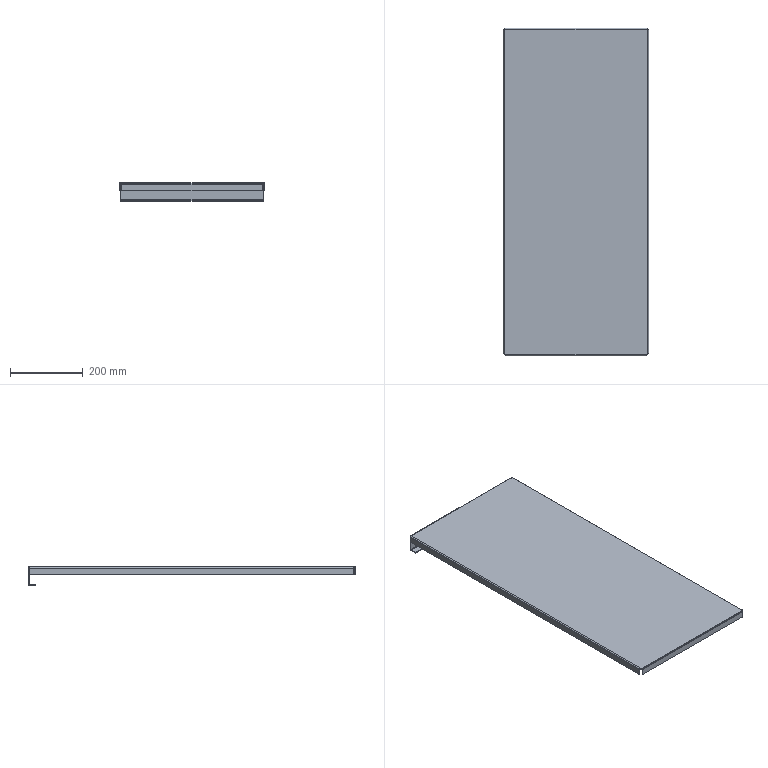Part | SolidWorks | features BaseBody 1 | 1 solid | 54 faces | box 398 x 898.5 x 50 mm | volume 1045766 mm3 | plane 44 | cylinder 10 | commonest cylinder face diameters 1.473 x5 6.473 x5
STEP:
#1=CARTESIAN_POINT('',(195.763,430.5,-47.5));
#2=VERTEX_POINT('',#1);
#3=CARTESIAN_POINT('',(-195.763,430.5,-47.5));
#4=VERTEX_POINT('',#3);
#5=CARTESIAN_POINT('',(-195.763,430.5,-47.5));
#6=DIRECTION('',(-1.,0.,0.));
#7=VECTOR('',#6,1000.);
#8=LINE('',#5,#7);
#9=EDGE_CURVE('',#2,#4,#8,.T.);
#10=ORIENTED_EDGE('',*,*,#9,.T.);
#11=CARTESIAN_POINT('',(-195.763,430.5,-50.));
#12=VERTEX_POINT('',#11);
#13=CARTESIAN_POINT('',(-195.763,430.5,-50.));
#14=DIRECTION('',(0.,0.,1.));
#15=VECTOR('',#14,1000.);
#16=LINE('',#13,#15);
#17=EDGE_CURVE('',#12,#4,#16,.T.);
#18=ORIENTED_EDGE('',*,*,#17,.F.);
#19=CARTESIAN_POINT('',(195.763,430.5,-50.));
#20=VERTEX_POINT('',#19);
#21=CARTESIAN_POINT('',(0.,430.5,-50.));
#22=DIRECTION('',(-1.,0.,0.));
#23=VECTOR('',#22,1000.);
#24=LINE('',#21,#23);
#25=EDGE_CURVE('',#20,#12,#24,.T.);
#26=ORIENTED_EDGE('',*,*,#25,.F.);
#27=CARTESIAN_POINT('',(195.763,430.5,-50.));
#28=DIRECTION('',(0.,0.,1.));
#29=VECTOR('',#28,1000.);
#30=LINE('',#27,#29);
#31=EDGE_CURVE('',#20,#2,#30,.T.);
#32=ORIENTED_EDGE('',*,*,#31,.T.);
#33=EDGE_LOOP('',(#10,#18,#26,#32));
#34=FACE_OUTER_BOUND('',#33,.T.);
#35=CARTESIAN_POINT('',(-195.763,430.5,-50.));
#36=DIRECTION('',(0.,1.,0.));
#37=DIRECTION('',(0.,0.,-1.));
#38=AXIS2_PLACEMENT_3D('',#35,#36,#37);
#39=PLANE('',#38);
#40=ADVANCED_FACE('',(#34),#39,.F.);
#41=CARTESIAN_POINT('',(195.763,447.263,-47.5));
#42=VERTEX_POINT('',#41);
#43=CARTESIAN_POINT('',(195.763,430.5,-47.5));
#44=DIRECTION('',(0.,-1.,0.));
#45=VECTOR('',#44,1000.);
#46=LINE('',#43,#45);
#47=EDGE_CURVE('',#42,#2,#46,.T.);
#48=ORIENTED_EDGE('',*,*,#47,.F.);
#49=CARTESIAN_POINT('',(-195.763,447.263,-47.5));
#50=VERTEX_POINT('',#49);
#51=CARTESIAN_POINT('',(-195.763,447.263,-47.5));
#52=DIRECTION('',(1.,0.,0.));
#53=VECTOR('',#52,1000.);
#54=LINE('',#51,#53);
#55=EDGE_CURVE('',#50,#42,#54,.T.);
#56=ORIENTED_EDGE('',*,*,#55,.F.);
#57=CARTESIAN_POINT('',(-195.763,448.,-47.5));
#58=DIRECTION('',(0.,1.,0.));
#59=VECTOR('',#58,1000.);
#60=LINE('',#57,#59);
#61=EDGE_CURVE('',#4,#50,#60,.T.);
#62=ORIENTED_EDGE('',*,*,#61,.F.);
#63=ORIENTED_EDGE('',*,*,#9,.F.);
#64=EDGE_LOOP('',(#48,#56,#62,#63));
#65=FACE_OUTER_BOUND('',#64,.T.);
#66=CARTESIAN_POINT('',(0.,0.,-47.5));
#67=DIRECTION('',(0.,0.,1.));
#68=DIRECTION('',(0.,-1.,0.));
#69=AXIS2_PLACEMENT_3D('',#66,#67,#68);
#70=PLANE('',#69);
#71=ADVANCED_FACE('',(#65),#70,.T.);
#72=CARTESIAN_POINT('',(195.763,447.263,-50.));
#73=VERTEX_POINT('',#72);
#74=CARTESIAN_POINT('',(-195.763,447.263,-50.));
#75=VERTEX_POINT('',#74);
#76=CARTESIAN_POINT('',(-195.763,447.263,-50.));
#77=DIRECTION('',(-1.,0.,0.));
#78=VECTOR('',#77,1000.);
#79=LINE('',#76,#78);
#80=EDGE_CURVE('',#73,#75,#79,.T.);
#81=ORIENTED_EDGE('',*,*,#80,.F.);
#82=CARTESIAN_POINT('',(195.763,0.,-50.));
#83=DIRECTION('',(0.,-1.,0.));
#84=VECTOR('',#83,1000.);
#85=LINE('',#82,#84);
#86=EDGE_CURVE('',#73,#20,#85,.T.);
#87=ORIENTED_EDGE('',*,*,#86,.T.);
#88=ORIENTED_EDGE('',*,*,#25,.T.);
#89=CARTESIAN_POINT('',(-195.763,0.,-50.));
#90=DIRECTION('',(0.,1.,0.));
#91=VECTOR('',#90,1000.);
#92=LINE('',#89,#91);
#93=EDGE_CURVE('',#12,#75,#92,.T.);
#94=ORIENTED_EDGE('',*,*,#93,.T.);
#95=EDGE_LOOP('',(#81,#87,#88,#94));
#96=FACE_OUTER_BOUND('',#95,.T.);
#97=CARTESIAN_POINT('',(0.,0.,-50.));
#98=DIRECTION('',(0.,0.,1.));
#99=DIRECTION('',(0.,-1.,0.));
#100=AXIS2_PLACEMENT_3D('',#97,#98,#99);
#101=PLANE('',#100);
#102=ADVANCED_FACE('',(#96),#101,.F.);
#103=CARTESIAN_POINT('',(-195.763,447.263,-50.));
#104=DIRECTION('',(0.,0.,-1.));
#105=VECTOR('',#104,1000.);
#106=LINE('',#103,#105);
#107=EDGE_CURVE('',#50,#75,#106,.T.);
#108=ORIENTED_EDGE('',*,*,#107,.T.);
#109=ORIENTED_EDGE('',*,*,#93,.F.);
#110=ORIENTED_EDGE('',*,*,#17,.T.);
#111=ORIENTED_EDGE('',*,*,#61,.T.);
#112=EDGE_LOOP('',(#108,#109,#110,#111));
#113=FACE_OUTER_BOUND('',#112,.T.);
#114=CARTESIAN_POINT('',(-195.763,448.,-50.));
#115=DIRECTION('',(1.,0.,0.));
#116=DIRECTION('',(0.,0.,-1.));
#117=AXIS2_PLACEMENT_3D('',#114,#115,#116);
#118=PLANE('',#117);
#119=ADVANCED_FACE('',(#113),#118,.F.);
#120=CARTESIAN_POINT('',(195.763,447.263,-47.5));
#121=DIRECTION('',(0.,0.,-1.));
#122=VECTOR('',#121,1000.);
#123=LINE('',#120,#122);
#124=EDGE_CURVE('',#42,#73,#123,.T.);
#125=ORIENTED_EDGE('',*,*,#124,.F.);
#126=ORIENTED_EDGE('',*,*,#47,.T.);
#127=ORIENTED_EDGE('',*,*,#31,.F.);
#128=ORIENTED_EDGE('',*,*,#86,.F.);
#129=EDGE_LOOP('',(#125,#126,#127,#128));
#130=FACE_OUTER_BOUND('',#129,.T.);
#131=CARTESIAN_POINT('',(195.763,430.5,-50.));
#132=DIRECTION('',(-1.,0.,0.));
#133=DIRECTION('',(0.,1.,0.));
#134=AXIS2_PLACEMENT_3D('',#131,#132,#133);
#135=PLANE('',#134);
#136=ADVANCED_FACE('',(#130),#135,.F.);
#137=CARTESIAN_POINT('',(195.763,448.,-46.763));
#138=VERTEX_POINT('',#137);
#139=CARTESIAN_POINT('',(-195.763,448.,-46.763));
#140=VERTEX_POINT('',#139);
#141=CARTESIAN_POINT('',(195.763,448.,-46.763));
#142=DIRECTION('',(-1.,0.,0.));
#143=VECTOR('',#142,1000.);
#144=LINE('',#141,#143);
#145=EDGE_CURVE('',#138,#140,#144,.T.);
#146=ORIENTED_EDGE('',*,*,#145,.T.);
#147=CARTESIAN_POINT('',(-195.763,447.263,-46.763));
#148=DIRECTION('',(-1.,0.,0.));
#149=DIRECTION('',(0.,0.,-1.));
#150=AXIS2_PLACEMENT_3D('',#147,#148,#149);
#151=CIRCLE('',#150,0.7366);
#152=EDGE_CURVE('',#140,#50,#151,.T.);
#153=ORIENTED_EDGE('',*,*,#152,.T.);
#154=ORIENTED_EDGE('',*,*,#55,.T.);
#155=CARTESIAN_POINT('',(195.763,447.263,-46.763));
#156=DIRECTION('',(1.,0.,0.));
#157=DIRECTION('',(0.,0.,-1.));
#158=AXIS2_PLACEMENT_3D('',#155,#156,#157);
#159=CIRCLE('',#158,0.7366);
#160=EDGE_CURVE('',#42,#138,#159,.T.);
#161=ORIENTED_EDGE('',*,*,#160,.T.);
#162=EDGE_LOOP('',(#146,#153,#154,#161));
#163=FACE_OUTER_BOUND('',#162,.T.);
#164=CARTESIAN_POINT('',(195.763,447.263,-46.763));
#165=DIRECTION('',(1.,0.,0.));
#166=DIRECTION('',(0.,0.,-1.));
#167=AXIS2_PLACEMENT_3D('',#164,#165,#166);
#168=CYLINDRICAL_SURFACE('',#167,0.7366);
#169=ADVANCED_FACE('',(#163),#168,.F.);
#170=CARTESIAN_POINT('',(195.763,450.5,-46.763));
#171=VERTEX_POINT('',#170);
#172=CARTESIAN_POINT('',(-195.763,450.5,-46.763));
#173=VERTEX_POINT('',#172);
#174=CARTESIAN_POINT('',(195.763,450.5,-46.763));
#175=DIRECTION('',(-1.,0.,0.));
#176=VECTOR('',#175,1000.);
#177=LINE('',#174,#176);
#178=EDGE_CURVE('',#171,#173,#177,.T.);
#179=ORIENTED_EDGE('',*,*,#178,.F.);
#180=CARTESIAN_POINT('',(195.763,447.263,-46.763));
#181=DIRECTION('',(1.,0.,0.));
#182=DIRECTION('',(0.,0.,-1.));
#183=AXIS2_PLACEMENT_3D('',#180,#181,#182);
#184=CIRCLE('',#183,3.237);
#185=EDGE_CURVE('',#73,#171,#184,.T.);
#186=ORIENTED_EDGE('',*,*,#185,.F.);
#187=ORIENTED_EDGE('',*,*,#80,.T.);
#188=CARTESIAN_POINT('',(-195.763,447.263,-46.763));
#189=DIRECTION('',(-1.,0.,0.));
#190=DIRECTION('',(0.,0.,-1.));
#191=AXIS2_PLACEMENT_3D('',#188,#189,#190);
#192=CIRCLE('',#191,3.237);
#193=EDGE_CURVE('',#173,#75,#192,.T.);
#194=ORIENTED_EDGE('',*,*,#193,.F.);
#195=EDGE_LOOP('',(#179,#186,#187,#194));
#196=FACE_OUTER_BOUND('',#195,.T.);
#197=CARTESIAN_POINT('',(195.763,447.263,-46.763));
#198=DIRECTION('',(1.,0.,0.));
#199=DIRECTION('',(0.,0.,-1.));
#200=AXIS2_PLACEMENT_3D('',#197,#198,#199);
#201=CYLINDRICAL_SURFACE('',#200,3.237);
#202=ADVANCED_FACE('',(#196),#201,.T.);
#203=ORIENTED_EDGE('',*,*,#160,.F.);
#204=ORIENTED_EDGE('',*,*,#124,.T.);
#205=ORIENTED_EDGE('',*,*,#185,.T.);
#206=CARTESIAN_POINT('',(195.763,448.,-46.763));
#207=DIRECTION('',(0.,1.,0.));
#208=VECTOR('',#207,1000.);
#209=LINE('',#206,#208);
#210=EDGE_CURVE('',#138,#171,#209,.T.);
#211=ORIENTED_EDGE('',*,*,#210,.F.);
#212=EDGE_LOOP('',(#203,#204,#205,#211));
#213=FACE_OUTER_BOUND('',#212,.T.);
#214=CARTESIAN_POINT('',(195.763,447.263,-46.763));
#215=DIRECTION('',(-1.,0.,0.));
#216=DIRECTION('',(0.,0.,1.));
#217=AXIS2_PLACEMENT_3D('',#214,#215,#216);
#218=PLANE('',#217);
#219=ADVANCED_FACE('',(#213),#218,.F.);
#220=ORIENTED_EDGE('',*,*,#107,.F.);
#221=ORIENTED_EDGE('',*,*,#152,.F.);
#222=CARTESIAN_POINT('',(-195.763,448.,-46.763));
#223=DIRECTION('',(0.,1.,0.));
#224=VECTOR('',#223,1000.);
#225=LINE('',#222,#224);
#226=EDGE_CURVE('',#140,#173,#225,.T.);
#227=ORIENTED_EDGE('',*,*,#226,.T.);
#228=ORIENTED_EDGE('',*,*,#193,.T.);
#229=EDGE_LOOP('',(#220,#221,#227,#228));
#230=FACE_OUTER_BOUND('',#229,.T.);
#231=CARTESIAN_POINT('',(-195.763,447.263,-46.763));
#232=DIRECTION('',(-1.,0.,0.));
#233=DIRECTION('',(0.,0.,1.));
#234=AXIS2_PLACEMENT_3D('',#231,#232,#233);
#235=PLANE('',#234);
#236=ADVANCED_FACE('',(#230),#235,.T.);
#237=CARTESIAN_POINT('',(195.763,447.263,-2.5));
#238=VERTEX_POINT('',#237);
#239=CARTESIAN_POINT('',(-195.763,447.263,-2.5));
#240=VERTEX_POINT('',#239);
#241=CARTESIAN_POINT('',(195.763,447.263,-2.5));
#242=DIRECTION('',(-1.,0.,0.));
#243=VECTOR('',#242,1000.);
#244=LINE('',#241,#243);
#245=EDGE_CURVE('',#238,#240,#244,.T.);
#246=ORIENTED_EDGE('',*,*,#245,.T.);
#247=CARTESIAN_POINT('',(-195.763,448.,-3.237));
#248=VERTEX_POINT('',#247);
#249=CARTESIAN_POINT('',(-195.763,447.263,-3.237));
#250=DIRECTION('',(-1.,0.,0.));
#251=DIRECTION('',(0.,0.,-1.));
#252=AXIS2_PLACEMENT_3D('',#249,#250,#251);
#253=CIRCLE('',#252,0.7366);
#254=EDGE_CURVE('',#240,#248,#253,.T.);
#255=ORIENTED_EDGE('',*,*,#254,.T.);
#256=CARTESIAN_POINT('',(195.763,448.,-3.237));
#257=VERTEX_POINT('',#256);
#258=CARTESIAN_POINT('',(-195.763,448.,-3.237));
#259=DIRECTION('',(1.,0.,0.));
#260=VECTOR('',#259,1000.);
#261=LINE('',#258,#260);
#262=EDGE_CURVE('',#248,#257,#261,.T.);
#263=ORIENTED_EDGE('',*,*,#262,.T.);
#264=CARTESIAN_POINT('',(195.763,447.263,-3.237));
#265=DIRECTION('',(1.,0.,0.));
#266=DIRECTION('',(0.,0.,-1.));
#267=AXIS2_PLACEMENT_3D('',#264,#265,#266);
#268=CIRCLE('',#267,0.7366);
#269=EDGE_CURVE('',#257,#238,#268,.T.);
#270=ORIENTED_EDGE('',*,*,#269,.T.);
#271=EDGE_LOOP('',(#246,#255,#263,#270));
#272=FACE_OUTER_BOUND('',#271,.T.);
#273=CARTESIAN_POINT('',(195.763,447.263,-3.237));
#274=DIRECTION('',(1.,0.,0.));
#275=DIRECTION('',(0.,1.,0.));
#276=AXIS2_PLACEMENT_3D('',#273,#274,#275);
#277=CYLINDRICAL_SURFACE('',#276,0.7366);
#278=ADVANCED_FACE('',(#272),#277,.F.);
#279=CARTESIAN_POINT('',(195.763,447.263,0.));
#280=VERTEX_POINT('',#279);
#281=CARTESIAN_POINT('',(-195.763,447.263,0.));
#282=VERTEX_POINT('',#281);
#283=CARTESIAN_POINT('',(195.763,447.263,0.));
#284=DIRECTION('',(-1.,0.,0.));
#285=VECTOR('',#284,1000.);
#286=LINE('',#283,#285);
#287=EDGE_CURVE('',#280,#282,#286,.T.);
#288=ORIENTED_EDGE('',*,*,#287,.F.);
#289=CARTESIAN_POINT('',(195.763,450.5,-3.237));
#290=VERTEX_POINT('',#289);
#291=CARTESIAN_POINT('',(195.763,447.263,-3.237));
#292=DIRECTION('',(1.,0.,0.));
#293=DIRECTION('',(0.,0.,-1.));
#294=AXIS2_PLACEMENT_3D('',#291,#292,#293);
#295=CIRCLE('',#294,3.237);
#296=EDGE_CURVE('',#290,#280,#295,.T.);
#297=ORIENTED_EDGE('',*,*,#296,.F.);
#298=CARTESIAN_POINT('',(-195.763,450.5,-3.237));
#299=VERTEX_POINT('',#298);
#300=CARTESIAN_POINT('',(0.,450.5,-3.237));
#301=DIRECTION('',(-1.,0.,0.));
#302=VECTOR('',#301,1000.);
#303=LINE('',#300,#302);
#304=EDGE_CURVE('',#290,#299,#303,.T.);
#305=ORIENTED_EDGE('',*,*,#304,.T.);
#306=CARTESIAN_POINT('',(-195.763,447.263,-3.237));
#307=DIRECTION('',(-1.,0.,0.));
#308=DIRECTION('',(0.,0.,-1.));
#309=AXIS2_PLACEMENT_3D('',#306,#307,#308);
#310=CIRCLE('',#309,3.237);
#311=EDGE_CURVE('',#282,#299,#310,.T.);
#312=ORIENTED_EDGE('',*,*,#311,.F.);
#313=EDGE_LOOP('',(#288,#297,#305,#312));
#314=FACE_OUTER_BOUND('',#313,.T.);
#315=CARTESIAN_POINT('',(195.763,447.263,-3.237));
#316=DIRECTION('',(1.,0.,0.));
#317=DIRECTION('',(0.,1.,0.));
#318=AXIS2_PLACEMENT_3D('',#315,#316,#317);
#319=CYLINDRICAL_SURFACE('',#318,3.237);
#320=ADVANCED_FACE('',(#314),#319,.T.);
#321=ORIENTED_EDGE('',*,*,#269,.F.);
#322=CARTESIAN_POINT('',(195.763,448.,-3.237));
#323=DIRECTION('',(0.,1.,0.));
#324=VECTOR('',#323,1000.);
#325=LINE('',#322,#324);
#326=EDGE_CURVE('',#257,#290,#325,.T.);
#327=ORIENTED_EDGE('',*,*,#326,.T.);
#328=ORIENTED_EDGE('',*,*,#296,.T.);
#329=CARTESIAN_POINT('',(195.763,447.263,-2.5));
#330=DIRECTION('',(0.,0.,1.));
#331=VECTOR('',#330,1000.);
#332=LINE('',#329,#331);
#333=EDGE_CURVE('',#238,#280,#332,.T.);
#334=ORIENTED_EDGE('',*,*,#333,.F.);
#335=EDGE_LOOP('',(#321,#327,#328,#334));
#336=FACE_OUTER_BOUND('',#335,.T.);
#337=CARTESIAN_POINT('',(195.763,447.263,-3.237));
#338=DIRECTION('',(-1.,0.,0.));
#339=DIRECTION('',(0.,0.,1.));
#340=AXIS2_PLACEMENT_3D('',#337,#338,#339);
#341=PLANE('',#340);
#342=ADVANCED_FACE('',(#336),#341,.F.);
#343=CARTESIAN_POINT('',(-195.763,448.,-3.237));
#344=DIRECTION('',(0.,1.,0.));
#345=VECTOR('',#344,1000.);
#346=LINE('',#343,#345);
#347=EDGE_CURVE('',#248,#299,#346,.T.);
#348=ORIENTED_EDGE('',*,*,#347,.F.);
#349=ORIENTED_EDGE('',*,*,#254,.F.);
#350=CARTESIAN_POINT('',(-195.763,447.263,-2.5));
#351=DIRECTION('',(0.,0.,1.));
#352=VECTOR('',#351,1000.);
#353=LINE('',#350,#352);
#354=EDGE_CURVE('',#240,#282,#353,.T.);
#355=ORIENTED_EDGE('',*,*,#354,.T.);
#356=ORIENTED_EDGE('',*,*,#311,.T.);
#357=EDGE_LOOP('',(#348,#349,#355,#356));
#358=FACE_OUTER_BOUND('',#357,.T.);
#359=CARTESIAN_POINT('',(-195.763,447.263,-3.237));
#360=DIRECTION('',(-1.,0.,0.));
#361=DIRECTION('',(0.,0.,1.));
#362=AXIS2_PLACEMENT_3D('',#359,#360,#361);
#363=PLANE('',#362);
#364=ADVANCED_FACE('',(#358),#363,.T.);
#365=CARTESIAN_POINT('',(-192.,-445.5,-20.));
#366=VERTEX_POINT('',#365);
#367=CARTESIAN_POINT('',(192.,-445.5,-20.));
#368=VERTEX_POINT('',#367);
#369=CARTESIAN_POINT('',(192.,-445.5,-20.));
#370=DIRECTION('',(1.,0.,0.));
#371=VECTOR('',#370,1000.);
#372=LINE('',#369,#371);
#373=EDGE_CURVE('',#366,#368,#372,.T.);
#374=ORIENTED_EDGE('',*,*,#373,.T.);
#375=CARTESIAN_POINT('',(192.,-448.,-20.));
#376=VERTEX_POINT('',#375);
#377=CARTESIAN_POINT('',(192.,-448.,-20.));
#378=DIRECTION('',(0.,1.,0.));
#379=VECTOR('',#378,1000.);
#380=LINE('',#377,#379);
#381=EDGE_CURVE('',#376,#368,#380,.T.);
#382=ORIENTED_EDGE('',*,*,#381,.F.);
#383=CARTESIAN_POINT('',(-192.,-448.,-20.));
#384=VERTEX_POINT('',#383);
#385=CARTESIAN_POINT('',(0.,-448.,-20.));
#386=DIRECTION('',(1.,0.,0.));
#387=VECTOR('',#386,1000.);
#388=LINE('',#385,#387);
#389=EDGE_CURVE('',#384,#376,#388,.T.);
#390=ORIENTED_EDGE('',*,*,#389,.F.);
#391=CARTESIAN_POINT('',(-192.,-448.,-20.));
#392=DIRECTION('',(0.,1.,0.));
#393=VECTOR('',#392,1000.);
#394=LINE('',#391,#393);
#395=EDGE_CURVE('',#384,#366,#394,.T.);
#396=ORIENTED_EDGE('',*,*,#395,.T.);
#397=EDGE_LOOP('',(#374,#382,#390,#396));
#398=FACE_OUTER_BOUND('',#397,.T.);
#399=CARTESIAN_POINT('',(192.,-448.,-20.));
#400=DIRECTION('',(0.,0.,1.));
#401=DIRECTION('',(0.,-1.,0.));
#402=AXIS2_PLACEMENT_3D('',#399,#400,#401);
#403=PLANE('',#402);
#404=ADVANCED_FACE('',(#398),#403,.F.);
#405=CARTESIAN_POINT('',(-192.,-445.5,-3.237));
#406=VERTEX_POINT('',#405);
#407=CARTESIAN_POINT('',(-192.,-445.5,-20.));
#408=DIRECTION('',(0.,0.,-1.));
#409=VECTOR('',#408,1000.);
#410=LINE('',#407,#409);
#411=EDGE_CURVE('',#406,#366,#410,.T.);
#412=ORIENTED_EDGE('',*,*,#411,.F.);
#413=CARTESIAN_POINT('',(192.,-445.5,-3.237));
#414=VERTEX_POINT('',#413);
#415=CARTESIAN_POINT('',(192.,-445.5,-3.237));
#416=DIRECTION('',(-1.,0.,0.));
#417=VECTOR('',#416,1000.);
#418=LINE('',#415,#417);
#419=EDGE_CURVE('',#414,#406,#418,.T.);
#420=ORIENTED_EDGE('',*,*,#419,.F.);
#421=CARTESIAN_POINT('',(192.,-445.5,-2.5));
#422=DIRECTION('',(0.,0.,1.));
#423=VECTOR('',#422,1000.);
#424=LINE('',#421,#423);
#425=EDGE_CURVE('',#368,#414,#424,.T.);
#426=ORIENTED_EDGE('',*,*,#425,.F.);
#427=ORIENTED_EDGE('',*,*,#373,.F.);
#428=EDGE_LOOP('',(#412,#420,#426,#427));
#429=FACE_OUTER_BOUND('',#428,.T.);
#430=CARTESIAN_POINT('',(0.,-445.5,0.));
#431=DIRECTION('',(0.,1.,0.));
#432=DIRECTION('',(0.,0.,-1.));
#433=AXIS2_PLACEMENT_3D('',#430,#431,#432);
#434=PLANE('',#433);
#435=ADVANCED_FACE('',(#429),#434,.T.);
#436=CARTESIAN_POINT('',(-192.,-448.,-3.237));
#437=VERTEX_POINT('',#436);
#438=CARTESIAN_POINT('',(192.,-448.,-3.237));
#439=VERTEX_POINT('',#438);
#440=CARTESIAN_POINT('',(192.,-448.,-3.237));
#441=DIRECTION('',(1.,0.,0.));
#442=VECTOR('',#441,1000.);
#443=LINE('',#440,#442);
#444=EDGE_CURVE('',#437,#439,#443,.T.);
#445=ORIENTED_EDGE('',*,*,#444,.F.);
#446=CARTESIAN_POINT('',(-192.,-448.,0.));
#447=DIRECTION('',(0.,0.,-1.));
#448=VECTOR('',#447,1000.);
#449=LINE('',#446,#448);
#450=EDGE_CURVE('',#437,#384,#449,.T.);
#451=ORIENTED_EDGE('',*,*,#450,.T.);
#452=ORIENTED_EDGE('',*,*,#389,.T.);
#453=CARTESIAN_POINT('',(192.,-448.,0.));
#454=DIRECTION('',(0.,0.,1.));
#455=VECTOR('',#454,1000.);
#456=LINE('',#453,#455);
#457=EDGE_CURVE('',#376,#439,#456,.T.);
#458=ORIENTED_EDGE('',*,*,#457,.T.);
#459=EDGE_LOOP('',(#445,#451,#452,#458));
#460=FACE_OUTER_BOUND('',#459,.T.);
#461=CARTESIAN_POINT('',(0.,-448.,0.));
#462=DIRECTION('',(0.,1.,0.));
#463=DIRECTION('',(0.,0.,-1.));
#464=AXIS2_PLACEMENT_3D('',#461,#462,#463);
#465=PLANE('',#464);
#466=ADVANCED_FACE('',(#460),#465,.F.);
#467=CARTESIAN_POINT('',(192.,-448.,-3.237));
#468=DIRECTION('',(0.,-1.,0.));
#469=VECTOR('',#468,1000.);
#470=LINE('',#467,#469);
#471=EDGE_CURVE('',#414,#439,#470,.T.);
#472=ORIENTED_EDGE('',*,*,#471,.T.);
#473=ORIENTED_EDGE('',*,*,#457,.F.);
#474=ORIENTED_EDGE('',*,*,#381,.T.);
#475=ORIENTED_EDGE('',*,*,#425,.T.);
#476=EDGE_LOOP('',(#472,#473,#474,#475));
#477=FACE_OUTER_BOUND('',#476,.T.);
#478=CARTESIAN_POINT('',(192.,-448.,-2.5));
#479=DIRECTION('',(-1.,0.,0.));
#480=DIRECTION('',(0.,0.,1.));
#481=AXIS2_PLACEMENT_3D('',#478,#479,#480);
#482=PLANE('',#481);
#483=ADVANCED_FACE('',(#477),#482,.F.);
#484=CARTESIAN_POINT('',(-192.,-445.5,-3.237));
#485=DIRECTION('',(0.,-1.,0.));
#486=VECTOR('',#485,1000.);
#487=LINE('',#484,#486);
#488=EDGE_CURVE('',#406,#437,#487,.T.);
#489=ORIENTED_EDGE('',*,*,#488,.F.);
#490=ORIENTED_EDGE('',*,*,#411,.T.);
#491=ORIENTED_EDGE('',*,*,#395,.F.);
#492=ORIENTED_EDGE('',*,*,#450,.F.);
#493=EDGE_LOOP('',(#489,#490,#491,#492));
#494=FACE_OUTER_BOUND('',#493,.T.);
#495=CARTESIAN_POINT('',(-192.,-448.,-20.));
#496=DIRECTION('',(1.,0.,0.));
#497=DIRECTION('',(0.,1.,0.));
#498=AXIS2_PLACEMENT_3D('',#495,#496,#497);
#499=PLANE('',#498);
#500=ADVANCED_FACE('',(#494),#499,.F.);
#501=CARTESIAN_POINT('',(-192.,-444.763,-2.5));
#502=VERTEX_POINT('',#501);
#503=CARTESIAN_POINT('',(192.,-444.763,-2.5));
#504=VERTEX_POINT('',#503);
#505=CARTESIAN_POINT('',(-192.,-444.763,-2.5));
#506=DIRECTION('',(1.,0.,0.));
#507=VECTOR('',#506,1000.);
#508=LINE('',#505,#507);
#509=EDGE_CURVE('',#502,#504,#508,.T.);
#510=ORIENTED_EDGE('',*,*,#509,.T.);
#511=CARTESIAN_POINT('',(192.,-444.763,-3.237));
#512=DIRECTION('',(1.,0.,0.));
#513=DIRECTION('',(0.,0.,1.));
#514=AXIS2_PLACEMENT_3D('',#511,#512,#513);
#515=CIRCLE('',#514,0.7366);
#516=EDGE_CURVE('',#504,#414,#515,.T.);
#517=ORIENTED_EDGE('',*,*,#516,.T.);
#518=ORIENTED_EDGE('',*,*,#419,.T.);
#519=CARTESIAN_POINT('',(-192.,-444.763,-3.237));
#520=DIRECTION('',(-1.,0.,0.));
#521=DIRECTION('',(0.,0.,1.));
#522=AXIS2_PLACEMENT_3D('',#519,#520,#521);
#523=CIRCLE('',#522,0.7366);
#524=EDGE_CURVE('',#406,#502,#523,.T.);
#525=ORIENTED_EDGE('',*,*,#524,.T.);
#526=EDGE_LOOP('',(#510,#517,#518,#525));
#527=FACE_OUTER_BOUND('',#526,.T.);
#528=CARTESIAN_POINT('',(-192.,-444.763,-3.237));
#529=DIRECTION('',(-1.,0.,0.));
#530=DIRECTION('',(0.,-1.,0.));
#531=AXIS2_PLACEMENT_3D('',#528,#529,#530);
#532=CYLINDRICAL_SURFACE('',#531,0.7366);
#533=ADVANCED_FACE('',(#527),#532,.F.);
#534=CARTESIAN_POINT('',(-192.,-444.763,0.));
#535=VERTEX_POINT('',#534);
#536=CARTESIAN_POINT('',(192.,-444.763,0.));
#537=VERTEX_POINT('',#536);
#538=CARTESIAN_POINT('',(-192.,-444.763,0.));
#539=DIRECTION('',(1.,0.,0.));
#540=VECTOR('',#539,1000.);
#541=LINE('',#538,#540);
#542=EDGE_CURVE('',#535,#537,#541,.T.);
#543=ORIENTED_EDGE('',*,*,#542,.F.);
#544=CARTESIAN_POINT('',(-192.,-447.915,-2.5));
#545=VERTEX_POINT('',#544);
#546=CARTESIAN_POINT('',(-192.,-444.763,-3.237));
#547=DIRECTION('',(-1.,0.,0.));
#548=DIRECTION('',(0.,0.,1.));
#549=AXIS2_PLACEMENT_3D('',#546,#547,#548);
#550=CIRCLE('',#549,3.237);
#551=EDGE_CURVE('',#545,#535,#550,.T.);
#552=ORIENTED_EDGE('',*,*,#551,.F.);
#553=CARTESIAN_POINT('',(-192.,-444.763,-3.237));
#554=DIRECTION('',(-1.,0.,0.));
#555=DIRECTION('',(0.,0.,1.));
#556=AXIS2_PLACEMENT_3D('',#553,#554,#555);
#557=CIRCLE('',#556,3.237);
#558=EDGE_CURVE('',#437,#545,#557,.T.);
#559=ORIENTED_EDGE('',*,*,#558,.F.);
#560=ORIENTED_EDGE('',*,*,#444,.T.);
#561=CARTESIAN_POINT('',(192.,-447.915,-2.5));
#562=VERTEX_POINT('',#561);
#563=CARTESIAN_POINT('',(192.,-444.763,-3.237));
#564=DIRECTION('',(1.,0.,0.));
#565=DIRECTION('',(0.,0.,1.));
#566=AXIS2_PLACEMENT_3D('',#563,#564,#565);
#567=CIRCLE('',#566,3.237);
#568=EDGE_CURVE('',#562,#439,#567,.T.);
#569=ORIENTED_EDGE('',*,*,#568,.F.);
#570=CARTESIAN_POINT('',(192.,-444.763,-3.237));
#571=DIRECTION('',(1.,0.,0.));
#572=DIRECTION('',(0.,0.,1.));
#573=AXIS2_PLACEMENT_3D('',#570,#571,#572);
#574=CIRCLE('',#573,3.237);
#575=EDGE_CURVE('',#537,#562,#574,.T.);
#576=ORIENTED_EDGE('',*,*,#575,.F.);
#577=EDGE_LOOP('',(#543,#552,#559,#560,#569,#576));
#578=FACE_OUTER_BOUND('',#577,.T.);
#579=CARTESIAN_POINT('',(-192.,-444.763,-3.237));
#580=DIRECTION('',(-1.,0.,0.));
#581=DIRECTION('',(0.,-1.,0.));
#582=AXIS2_PLACEMENT_3D('',#579,#580,#581);
#583=CYLINDRICAL_SURFACE('',#582,3.237);
#584=ADVANCED_FACE('',(#578),#583,.T.);
#585=ORIENTED_EDGE('',*,*,#558,.T.);
#586=CARTESIAN_POINT('',(-192.,-448.,-2.5));
#587=DIRECTION('',(0.,1.,0.));
#588=VECTOR('',#587,1000.);
#589=LINE('',#586,#588);
#590=EDGE_CURVE('',#545,#502,#589,.T.);
#591=ORIENTED_EDGE('',*,*,#590,.T.);
#592=ORIENTED_EDGE('',*,*,#524,.F.);
#593=ORIENTED_EDGE('',*,*,#488,.T.);
#594=EDGE_LOOP('',(#585,#591,#592,#593));
#595=FACE_OUTER_BOUND('',#594,.T.);
#596=CARTESIAN_POINT('',(-192.,-444.763,-3.237));
#597=DIRECTION('',(1.,0.,0.));
#598=DIRECTION('',(0.,1.,0.));
#599=AXIS2_PLACEMENT_3D('',#596,#597,#598);
#600=PLANE('',#599);
#601=ADVANCED_FACE('',(#595),#600,.F.);
#602=ORIENTED_EDGE('',*,*,#516,.F.);
#603=CARTESIAN_POINT('',(192.,-444.763,-2.5));
#604=DIRECTION('',(0.,-1.,0.));
#605=VECTOR('',#604,1000.);
#606=LINE('',#603,#605);
#607=EDGE_CURVE('',#504,#562,#606,.T.);
#608=ORIENTED_EDGE('',*,*,#607,.T.);
#609=ORIENTED_EDGE('',*,*,#568,.T.);
#610=ORIENTED_EDGE('',*,*,#471,.F.);
#611=EDGE_LOOP('',(#602,#608,#609,#610));
#612=FACE_OUTER_BOUND('',#611,.T.);
#613=CARTESIAN_POINT('',(192.,-444.763,-3.237));
#614=DIRECTION('',(1.,0.,0.));
#615=DIRECTION('',(0.,1.,0.));
#616=AXIS2_PLACEMENT_3D('',#613,#614,#615);
#617=PLANE('',#616);
#618=ADVANCED_FACE('',(#612),#617,.T.);
#619=CARTESIAN_POINT('',(196.5,-441.,-20.));
#620=VERTEX_POINT('',#619);
#621=CARTESIAN_POINT('',(196.5,448.,-20.));
#622=VERTEX_POINT('',#621);
#623=CARTESIAN_POINT('',(196.5,448.,-20.));
#624=DIRECTION('',(0.,1.,0.));
#625=VECTOR('',#624,1000.);
#626=LINE('',#623,#625);
#627=EDGE_CURVE('',#620,#622,#626,.T.);
#628=ORIENTED_EDGE('',*,*,#627,.T.);
#629=CARTESIAN_POINT('',(199.,448.,-20.));
#630=VERTEX_POINT('',#629);
#631=CARTESIAN_POINT('',(199.,448.,-20.));
#632=DIRECTION('',(-1.,0.,0.));
#633=VECTOR('',#632,1000.);
#634=LINE('',#631,#633);
#635=EDGE_CURVE('',#630,#622,#634,.T.);
#636=ORIENTED_EDGE('',*,*,#635,.F.);
#637=CARTESIAN_POINT('',(199.,-441.,-20.));
#638=VERTEX_POINT('',#637);
#639=CARTESIAN_POINT('',(199.,0.,-20.));
#640=DIRECTION('',(0.,1.,0.));
#641=VECTOR('',#640,1000.);
#642=LINE('',#639,#641);
#643=EDGE_CURVE('',#638,#630,#642,.T.);
#644=ORIENTED_EDGE('',*,*,#643,.F.);
#645=CARTESIAN_POINT('',(199.,-441.,-20.));
#646=DIRECTION('',(-1.,0.,0.));
#647=VECTOR('',#646,1000.);
#648=LINE('',#645,#647);
#649=EDGE_CURVE('',#638,#620,#648,.T.);
#650=ORIENTED_EDGE('',*,*,#649,.T.);
#651=EDGE_LOOP('',(#628,#636,#644,#650));
#652=FACE_OUTER_BOUND('',#651,.T.);
#653=CARTESIAN_POINT('',(199.,448.,-20.));
#654=DIRECTION('',(0.,0.,1.));
#655=DIRECTION('',(1.,0.,0.));
#656=AXIS2_PLACEMENT_3D('',#653,#654,#655);
#657=PLANE('',#656);
#658=ADVANCED_FACE('',(#652),#657,.F.);
#659=CARTESIAN_POINT('',(196.5,-441.,-3.237));
#660=VERTEX_POINT('',#659);
#661=CARTESIAN_POINT('',(196.5,-441.,-20.));
#662=DIRECTION('',(0.,0.,-1.));
#663=VECTOR('',#662,1000.);
#664=LINE('',#661,#663);
#665=EDGE_CURVE('',#660,#620,#664,.T.);
#666=ORIENTED_EDGE('',*,*,#665,.F.);
#667=CARTESIAN_POINT('',(196.5,447.263,-3.237));
#668=VERTEX_POINT('',#667);
#669=CARTESIAN_POINT('',(196.5,448.,-3.237));
#670=DIRECTION('',(0.,-1.,0.));
#671=VECTOR('',#670,1000.);
#672=LINE('',#669,#671);
#673=EDGE_CURVE('',#668,#660,#672,.T.);
#674=ORIENTED_EDGE('',*,*,#673,.F.);
#675=CARTESIAN_POINT('',(196.5,448.,-3.237));
#676=VERTEX_POINT('',#675);
#677=CARTESIAN_POINT('',(196.5,448.,-3.237));
#678=DIRECTION('',(0.,-1.,0.));
#679=VECTOR('',#678,1000.);
#680=LINE('',#677,#679);
#681=EDGE_CURVE('',#676,#668,#680,.T.);
#682=ORIENTED_EDGE('',*,*,#681,.F.);
#683=CARTESIAN_POINT('',(196.5,448.,-2.5));
#684=DIRECTION('',(0.,0.,1.));
#685=VECTOR('',#684,1000.);
#686=LINE('',#683,#685);
#687=EDGE_CURVE('',#622,#676,#686,.T.);
#688=ORIENTED_EDGE('',*,*,#687,.F.);
#689=ORIENTED_EDGE('',*,*,#627,.F.);
#690=EDGE_LOOP('',(#666,#674,#682,#688,#689));
#691=FACE_OUTER_BOUND('',#690,.T.);
#692=CARTESIAN_POINT('',(196.5,0.,0.));
#693=DIRECTION('',(-1.,0.,0.));
#694=DIRECTION('',(0.,0.,1.));
#695=AXIS2_PLACEMENT_3D('',#692,#693,#694);
#696=PLANE('',#695);
#697=ADVANCED_FACE('',(#691),#696,.T.);
#698=CARTESIAN_POINT('',(199.,-441.,-3.237));
#699=VERTEX_POINT('',#698);
#700=CARTESIAN_POINT('',(199.,447.263,-3.237));
#701=VERTEX_POINT('',#700);
#702=CARTESIAN_POINT('',(199.,448.,-3.237));
#703=DIRECTION('',(0.,1.,0.));
#704=VECTOR('',#703,1000.);
#705=LINE('',#702,#704);
#706=EDGE_CURVE('',#699,#701,#705,.T.);
#707=ORIENTED_EDGE('',*,*,#706,.F.);
#708=CARTESIAN_POINT('',(199.,-441.,0.));
#709=DIRECTION('',(0.,0.,-1.));
#710=VECTOR('',#709,1000.);
#711=LINE('',#708,#710);
#712=EDGE_CURVE('',#699,#638,#711,.T.);
#713=ORIENTED_EDGE('',*,*,#712,.T.);
#714=ORIENTED_EDGE('',*,*,#643,.T.);
#715=CARTESIAN_POINT('',(199.,448.,-3.237));
#716=VERTEX_POINT('',#715);
#717=CARTESIAN_POINT('',(199.,448.,0.));
#718=DIRECTION('',(0.,0.,1.));
#719=VECTOR('',#718,1000.);
#720=LINE('',#717,#719);
#721=EDGE_CURVE('',#630,#716,#720,.T.);
#722=ORIENTED_EDGE('',*,*,#721,.T.);
#723=CARTESIAN_POINT('',(199.,448.,-3.237));
#724=DIRECTION('',(0.,1.,0.));
#725=VECTOR('',#724,1000.);
#726=LINE('',#723,#725);
#727=EDGE_CURVE('',#701,#716,#726,.T.);
#728=ORIENTED_EDGE('',*,*,#727,.F.);
#729=EDGE_LOOP('',(#707,#713,#714,#722,#728));
#730=FACE_OUTER_BOUND('',#729,.T.);
#731=CARTESIAN_POINT('',(199.,0.,0.));
#732=DIRECTION('',(-1.,0.,0.));
#733=DIRECTION('',(0.,0.,1.));
#734=AXIS2_PLACEMENT_3D('',#731,#732,#733);
#735=PLANE('',#734);
#736=ADVANCED_FACE('',(#730),#735,.F.);
#737=CARTESIAN_POINT('',(199.,448.,-3.237));
#738=DIRECTION('',(1.,0.,0.));
#739=VECTOR('',#738,1000.);
#740=LINE('',#737,#739);
#741=EDGE_CURVE('',#676,#716,#740,.T.);
#742=ORIENTED_EDGE('',*,*,#741,.T.);
#743=ORIENTED_EDGE('',*,*,#721,.F.);
#744=ORIENTED_EDGE('',*,*,#635,.T.);
#745=ORIENTED_EDGE('',*,*,#687,.T.);
#746=EDGE_LOOP('',(#742,#743,#744,#745));
#747=FACE_OUTER_BOUND('',#746,.T.);
#748=CARTESIAN_POINT('',(199.,448.,-2.5));
#749=DIRECTION('',(0.,-1.,0.));
#750=DIRECTION('',(0.,0.,-1.));
#751=AXIS2_PLACEMENT_3D('',#748,#749,#750);
#752=PLANE('',#751);
#753=ADVANCED_FACE('',(#747),#752,.F.);
#754=CARTESIAN_POINT('',(196.5,-441.,-3.237));
#755=DIRECTION('',(1.,0.,0.));
#756=VECTOR('',#755,1000.);
#757=LINE('',#754,#756);
#758=EDGE_CURVE('',#660,#699,#757,.T.);
#759=ORIENTED_EDGE('',*,*,#758,.F.);
#760=ORIENTED_EDGE('',*,*,#665,.T.);
#761=ORIENTED_EDGE('',*,*,#649,.F.);
#762=ORIENTED_EDGE('',*,*,#712,.F.);
#763=EDGE_LOOP('',(#759,#760,#761,#762));
#764=FACE_OUTER_BOUND('',#763,.T.);
#765=CARTESIAN_POINT('',(199.,-441.,-20.));
#766=DIRECTION('',(0.,1.,0.));
#767=DIRECTION('',(0.,0.,-1.));
#768=AXIS2_PLACEMENT_3D('',#765,#766,#767);
#769=PLANE('',#768);
#770=ADVANCED_FACE('',(#764),#769,.F.);
#771=CARTESIAN_POINT('',(195.763,447.263,-3.237));
#772=DIRECTION('',(0.,-1.,0.));
#773=DIRECTION('',(0.,0.,1.));
#774=AXIS2_PLACEMENT_3D('',#771,#772,#773);
#775=CIRCLE('',#774,0.7366);
#776=EDGE_CURVE('',#668,#238,#775,.T.);
#777=ORIENTED_EDGE('',*,*,#776,.F.);
#778=ORIENTED_EDGE('',*,*,#673,.T.);
#779=CARTESIAN_POINT('',(195.763,-441.,-2.5));
#780=VERTEX_POINT('',#779);
#781=CARTESIAN_POINT('',(195.763,-441.,-3.237));
#782=DIRECTION('',(0.,-1.,0.));
#783=DIRECTION('',(0.,0.,-1.));
#784=AXIS2_PLACEMENT_3D('',#781,#782,#783);
#785=CIRCLE('',#784,0.7366);
#786=EDGE_CURVE('',#660,#780,#785,.T.);
#787=ORIENTED_EDGE('',*,*,#786,.T.);
#788=CARTESIAN_POINT('',(195.763,-441.,-2.5));
#789=DIRECTION('',(0.,1.,0.));
#790=VECTOR('',#789,1000.);
#791=LINE('',#788,#790);
#792=EDGE_CURVE('',#780,#238,#791,.T.);
#793=ORIENTED_EDGE('',*,*,#792,.T.);
#794=EDGE_LOOP('',(#777,#778,#787,#793));
#795=FACE_OUTER_BOUND('',#794,.T.);
#796=CARTESIAN_POINT('',(195.763,-441.,-3.237));
#797=DIRECTION('',(0.,-1.,0.));
#798=DIRECTION('',(1.,0.,0.));
#799=AXIS2_PLACEMENT_3D('',#796,#797,#798);
#800=CYLINDRICAL_SURFACE('',#799,0.7366);
#801=ADVANCED_FACE('',(#795),#800,.F.);
#802=CARTESIAN_POINT('',(195.763,447.263,-3.237));
#803=DIRECTION('',(0.,-1.,0.));
#804=DIRECTION('',(0.,0.,1.));
#805=AXIS2_PLACEMENT_3D('',#802,#803,#804);
#806=CIRCLE('',#805,3.237);
#807=EDGE_CURVE('',#701,#280,#806,.T.);
#808=ORIENTED_EDGE('',*,*,#807,.F.);
#809=CARTESIAN_POINT('',(199.,447.263,-3.237));
#810=DIRECTION('',(-1.,0.,0.));
#811=VECTOR('',#810,1000.);
#812=LINE('',#809,#811);
#813=EDGE_CURVE('',#701,#668,#812,.T.);
#814=ORIENTED_EDGE('',*,*,#813,.T.);
#815=ORIENTED_EDGE('',*,*,#776,.T.);
#816=ORIENTED_EDGE('',*,*,#333,.T.);
#817=EDGE_LOOP('',(#808,#814,#815,#816));
#818=FACE_OUTER_BOUND('',#817,.T.);
#819=CARTESIAN_POINT('',(195.763,447.263,-3.237));
#820=DIRECTION('',(0.,1.,0.));
#821=DIRECTION('',(1.,0.,0.));
#822=AXIS2_PLACEMENT_3D('',#819,#820,#821);
#823=PLANE('',#822);
#824=ADVANCED_FACE('',(#818),#823,.T.);
#825=CARTESIAN_POINT('',(198.915,-441.,-2.5));
#826=VERTEX_POINT('',#825);
#827=CARTESIAN_POINT('',(195.763,-441.,-3.237));
#828=DIRECTION('',(0.,-1.,0.));
#829=DIRECTION('',(0.,0.,-1.));
#830=AXIS2_PLACEMENT_3D('',#827,#828,#829);
#831=CIRCLE('',#830,3.237);
#832=EDGE_CURVE('',#699,#826,#831,.T.);
#833=ORIENTED_EDGE('',*,*,#832,.T.);
#834=CARTESIAN_POINT('',(199.,-441.,-2.5));
#835=DIRECTION('',(-1.,0.,0.));
#836=VECTOR('',#835,1000.);
#837=LINE('',#834,#836);
#838=EDGE_CURVE('',#826,#780,#837,.T.);
#839=ORIENTED_EDGE('',*,*,#838,.T.);
#840=ORIENTED_EDGE('',*,*,#786,.F.);
#841=ORIENTED_EDGE('',*,*,#758,.T.);
#842=EDGE_LOOP('',(#833,#839,#840,#841));
#843=FACE_OUTER_BOUND('',#842,.T.);
#844=CARTESIAN_POINT('',(195.763,-441.,-3.237));
#845=DIRECTION('',(0.,1.,0.));
#846=DIRECTION('',(1.,0.,0.));
#847=AXIS2_PLACEMENT_3D('',#844,#845,#846);
#848=PLANE('',#847);
#849=ADVANCED_FACE('',(#843),#848,.F.);
#850=CARTESIAN_POINT('',(-196.5,448.,-20.));
#851=VERTEX_POINT('',#850);
#852=CARTESIAN_POINT('',(-196.5,-441.,-20.));
#853=VERTEX_POINT('',#852);
#854=CARTESIAN_POINT('',(-196.5,-441.,-20.));
#855=DIRECTION('',(0.,-1.,0.));
#856=VECTOR('',#855,1000.);
#857=LINE('',#854,#856);
#858=EDGE_CURVE('',#851,#853,#857,.T.);
#859=ORIENTED_EDGE('',*,*,#858,.T.);
#860=CARTESIAN_POINT('',(-199.,-441.,-20.));
#861=VERTEX_POINT('',#860);
#862=CARTESIAN_POINT('',(-199.,-441.,-20.));
#863=DIRECTION('',(1.,0.,0.));
#864=VECTOR('',#863,1000.);
#865=LINE('',#862,#864);
#866=EDGE_CURVE('',#861,#853,#865,.T.);
#867=ORIENTED_EDGE('',*,*,#866,.F.);
#868=CARTESIAN_POINT('',(-199.,448.,-20.));
#869=VERTEX_POINT('',#868);
#870=CARTESIAN_POINT('',(-199.,0.,-20.));
#871=DIRECTION('',(0.,-1.,0.));
#872=VECTOR('',#871,1000.);
#873=LINE('',#870,#872);
#874=EDGE_CURVE('',#869,#861,#873,.T.);
#875=ORIENTED_EDGE('',*,*,#874,.F.);
#876=CARTESIAN_POINT('',(-199.,448.,-20.));
#877=DIRECTION('',(1.,0.,0.));
#878=VECTOR('',#877,1000.);
#879=LINE('',#876,#878);
#880=EDGE_CURVE('',#869,#851,#879,.T.);
#881=ORIENTED_EDGE('',*,*,#880,.T.);
#882=EDGE_LOOP('',(#859,#867,#875,#881));
#883=FACE_OUTER_BOUND('',#882,.T.);
#884=CARTESIAN_POINT('',(-199.,-441.,-20.));
#885=DIRECTION('',(0.,0.,1.));
#886=DIRECTION('',(1.,0.,0.));
#887=AXIS2_PLACEMENT_3D('',#884,#885,#886);
#888=PLANE('',#887);
#889=ADVANCED_FACE('',(#883),#888,.F.);
#890=CARTESIAN_POINT('',(-196.5,448.,-3.237));
#891=VERTEX_POINT('',#890);
#892=CARTESIAN_POINT('',(-196.5,448.,-20.));
#893=DIRECTION('',(0.,0.,-1.));
#894=VECTOR('',#893,1000.);
#895=LINE('',#892,#894);
#896=EDGE_CURVE('',#891,#851,#895,.T.);
#897=ORIENTED_EDGE('',*,*,#896,.F.);
#898=CARTESIAN_POINT('',(-196.5,447.263,-3.237));
#899=VERTEX_POINT('',#898);
#900=CARTESIAN_POINT('',(-196.5,-441.,-3.237));
#901=DIRECTION('',(0.,1.,0.));
#902=VECTOR('',#901,1000.);
#903=LINE('',#900,#902);
#904=EDGE_CURVE('',#899,#891,#903,.T.);
#905=ORIENTED_EDGE('',*,*,#904,.F.);
#906=CARTESIAN_POINT('',(-196.5,-441.,-3.237));
#907=VERTEX_POINT('',#906);
#908=CARTESIAN_POINT('',(-196.5,-441.,-3.237));
#909=DIRECTION('',(0.,1.,0.));
#910=VECTOR('',#909,1000.);
#911=LINE('',#908,#910);
#912=EDGE_CURVE('',#907,#899,#911,.T.);
#913=ORIENTED_EDGE('',*,*,#912,.F.);
#914=CARTESIAN_POINT('',(-196.5,-441.,-2.5));
#915=DIRECTION('',(0.,0.,1.));
#916=VECTOR('',#915,1000.);
#917=LINE('',#914,#916);
#918=EDGE_CURVE('',#853,#907,#917,.T.);
#919=ORIENTED_EDGE('',*,*,#918,.F.);
#920=ORIENTED_EDGE('',*,*,#858,.F.);
#921=EDGE_LOOP('',(#897,#905,#913,#919,#920));
#922=FACE_OUTER_BOUND('',#921,.T.);
#923=CARTESIAN_POINT('',(-196.5,0.,0.));
#924=DIRECTION('',(1.,0.,0.));
#925=DIRECTION('',(0.,0.,-1.));
#926=AXIS2_PLACEMENT_3D('',#923,#924,#925);
#927=PLANE('',#926);
#928=ADVANCED_FACE('',(#922),#927,.T.);
#929=CARTESIAN_POINT('',(-199.,448.,-3.237));
#930=VERTEX_POINT('',#929);
#931=CARTESIAN_POINT('',(-199.,447.263,-3.237));
#932=VERTEX_POINT('',#931);
#933=CARTESIAN_POINT('',(-199.,-441.,-3.237));
#934=DIRECTION('',(0.,-1.,0.));
#935=VECTOR('',#934,1000.);
#936=LINE('',#933,#935);
#937=EDGE_CURVE('',#930,#932,#936,.T.);
#938=ORIENTED_EDGE('',*,*,#937,.F.);
#939=CARTESIAN_POINT('',(-199.,448.,0.));
#940=DIRECTION('',(0.,0.,-1.));
#941=VECTOR('',#940,1000.);
#942=LINE('',#939,#941);
#943=EDGE_CURVE('',#930,#869,#942,.T.);
#944=ORIENTED_EDGE('',*,*,#943,.T.);
#945=ORIENTED_EDGE('',*,*,#874,.T.);
#946=CARTESIAN_POINT('',(-199.,-441.,-3.237));
#947=VERTEX_POINT('',#946);
#948=CARTESIAN_POINT('',(-199.,-441.,0.));
#949=DIRECTION('',(0.,0.,1.));
#950=VECTOR('',#949,1000.);
#951=LINE('',#948,#950);
#952=EDGE_CURVE('',#861,#947,#951,.T.);
#953=ORIENTED_EDGE('',*,*,#952,.T.);
#954=CARTESIAN_POINT('',(-199.,-441.,-3.237));
#955=DIRECTION('',(0.,-1.,0.));
#956=VECTOR('',#955,1000.);
#957=LINE('',#954,#956);
#958=EDGE_CURVE('',#932,#947,#957,.T.);
#959=ORIENTED_EDGE('',*,*,#958,.F.);
#960=EDGE_LOOP('',(#938,#944,#945,#953,#959));
#961=FACE_OUTER_BOUND('',#960,.T.);
#962=CARTESIAN_POINT('',(-199.,0.,0.));
#963=DIRECTION('',(1.,0.,0.));
#964=DIRECTION('',(0.,0.,-1.));
#965=AXIS2_PLACEMENT_3D('',#962,#963,#964);
#966=PLANE('',#965);
#967=ADVANCED_FACE('',(#961),#966,.F.);
#968=CARTESIAN_POINT('',(-199.,-441.,-3.237));
#969=DIRECTION('',(-1.,0.,0.));
#970=VECTOR('',#969,1000.);
#971=LINE('',#968,#970);
#972=EDGE_CURVE('',#907,#947,#971,.T.);
#973=ORIENTED_EDGE('',*,*,#972,.T.);
#974=ORIENTED_EDGE('',*,*,#952,.F.);
#975=ORIENTED_EDGE('',*,*,#866,.T.);
#976=ORIENTED_EDGE('',*,*,#918,.T.);
#977=EDGE_LOOP('',(#973,#974,#975,#976));
#978=FACE_OUTER_BOUND('',#977,.T.);
#979=CARTESIAN_POINT('',(-199.,-441.,-2.5));
#980=DIRECTION('',(0.,1.,0.));
#981=DIRECTION('',(1.,0.,0.));
#982=AXIS2_PLACEMENT_3D('',#979,#980,#981);
#983=PLANE('',#982);
#984=ADVANCED_FACE('',(#978),#983,.F.);
#985=CARTESIAN_POINT('',(-196.5,448.,-3.237));
#986=DIRECTION('',(-1.,0.,0.));
#987=VECTOR('',#986,1000.);
#988=LINE('',#985,#987);
#989=EDGE_CURVE('',#891,#930,#988,.T.);
#990=ORIENTED_EDGE('',*,*,#989,.F.);
#991=ORIENTED_EDGE('',*,*,#896,.T.);
#992=ORIENTED_EDGE('',*,*,#880,.F.);
#993=ORIENTED_EDGE('',*,*,#943,.F.);
#994=EDGE_LOOP('',(#990,#991,#992,#993));
#995=FACE_OUTER_BOUND('',#994,.T.);
#996=CARTESIAN_POINT('',(-199.,448.,-20.));
#997=DIRECTION('',(0.,-1.,0.));
#998=DIRECTION('',(0.,0.,-1.));
#999=AXIS2_PLACEMENT_3D('',#996,#997,#998);
#1000=PLANE('',#999);
#1001=ADVANCED_FACE('',(#995),#1000,.F.);
#1002=CARTESIAN_POINT('',(-195.763,447.263,-3.237));
#1003=DIRECTION('',(0.,-1.,0.));
#1004=DIRECTION('',(0.,0.,1.));
#1005=AXIS2_PLACEMENT_3D('',#1002,#1003,#1004);
#1006=CIRCLE('',#1005,0.7366);
#1007=EDGE_CURVE('',#240,#899,#1006,.T.);
#1008=ORIENTED_EDGE('',*,*,#1007,.F.);
#1009=CARTESIAN_POINT('',(-195.763,-441.,-2.5));
#1010=VERTEX_POINT('',#1009);
#1011=CARTESIAN_POINT('',(-195.763,448.,-2.5));
#1012=DIRECTION('',(0.,-1.,0.));
#1013=VECTOR('',#1012,1000.);
#1014=LINE('',#1011,#1013);
#1015=EDGE_CURVE('',#240,#1010,#1014,.T.);
#1016=ORIENTED_EDGE('',*,*,#1015,.T.);
#1017=CARTESIAN_POINT('',(-195.763,-441.,-3.237));
#1018=DIRECTION('',(0.,-1.,0.));
#1019=DIRECTION('',(0.,0.,1.));
#1020=AXIS2_PLACEMENT_3D('',#1017,#1018,#1019);
#1021=CIRCLE('',#1020,0.7366);
#1022=EDGE_CURVE('',#1010,#907,#1021,.T.);
#1023=ORIENTED_EDGE('',*,*,#1022,.T.);
#1024=ORIENTED_EDGE('',*,*,#912,.T.);
#1025=EDGE_LOOP('',(#1008,#1016,#1023,#1024));
#1026=FACE_OUTER_BOUND('',#1025,.T.);
#1027=CARTESIAN_POINT('',(-195.763,448.,-3.237));
#1028=DIRECTION('',(0.,1.,0.));
#1029=DIRECTION('',(-1.,0.,0.));
#1030=AXIS2_PLACEMENT_3D('',#1027,#1028,#1029);
#1031=CYLINDRICAL_SURFACE('',#1030,0.7366);
#1032=ADVANCED_FACE('',(#1026),#1031,.F.);
#1033=ORIENTED_EDGE('',*,*,#1022,.F.);
#1034=CARTESIAN_POINT('',(-198.915,-441.,-2.5));
#1035=VERTEX_POINT('',#1034);
#1036=CARTESIAN_POINT('',(-195.763,-441.,-2.5));
#1037=DIRECTION('',(-1.,0.,0.));
#1038=VECTOR('',#1037,1000.);
#1039=LINE('',#1036,#1038);
#1040=EDGE_CURVE('',#1010,#1035,#1039,.T.);
#1041=ORIENTED_EDGE('',*,*,#1040,.T.);
#1042=CARTESIAN_POINT('',(-195.763,-441.,-3.237));
#1043=DIRECTION('',(0.,-1.,0.));
#1044=DIRECTION('',(0.,0.,1.));
#1045=AXIS2_PLACEMENT_3D('',#1042,#1043,#1044);
#1046=CIRCLE('',#1045,3.237);
#1047=EDGE_CURVE('',#1035,#947,#1046,.T.);
#1048=ORIENTED_EDGE('',*,*,#1047,.T.);
#1049=ORIENTED_EDGE('',*,*,#972,.F.);
#1050=EDGE_LOOP('',(#1033,#1041,#1048,#1049));
#1051=FACE_OUTER_BOUND('',#1050,.T.);
#1052=CARTESIAN_POINT('',(-195.763,-441.,-3.237));
#1053=DIRECTION('',(0.,-1.,0.));
#1054=DIRECTION('',(0.,0.,-1.));
#1055=AXIS2_PLACEMENT_3D('',#1052,#1053,#1054);
#1056=PLANE('',#1055);
#1057=ADVANCED_FACE('',(#1051),#1056,.T.);
#1058=CARTESIAN_POINT('',(199.,-441.,-2.5));
#1059=VERTEX_POINT('',#1058);
#1060=CARTESIAN_POINT('',(192.,-448.,-2.5));
#1061=VERTEX_POINT('',#1060);
#1062=CARTESIAN_POINT('',(320.,-320.,-2.5));
#1063=DIRECTION('',(-0.7071,-0.7071,0.));
#1064=VECTOR('',#1063,1000.);
#1065=LINE('',#1062,#1064);
#1066=EDGE_CURVE('',#1059,#1061,#1065,.T.);
#1067=ORIENTED_EDGE('',*,*,#1066,.F.);
#1068=CARTESIAN_POINT('',(199.,-441.,0.));
#1069=VERTEX_POINT('',#1068);
#1070=CARTESIAN_POINT('',(199.,-441.,-2.5));
#1071=DIRECTION('',(0.,0.,-1.));
#1072=VECTOR('',#1071,1000.);
#1073=LINE('',#1070,#1072);
#1074=EDGE_CURVE('',#1069,#1059,#1073,.T.);
#1075=ORIENTED_EDGE('',*,*,#1074,.F.);
#1076=CARTESIAN_POINT('',(192.,-448.,0.));
#1077=VERTEX_POINT('',#1076);
#1078=CARTESIAN_POINT('',(192.,-448.,0.));
#1079=DIRECTION('',(0.7071,0.7071,0.));
#1080=VECTOR('',#1079,1000.);
#1081=LINE('',#1078,#1080);
#1082=EDGE_CURVE('',#1077,#1069,#1081,.T.);
#1083=ORIENTED_EDGE('',*,*,#1082,.F.);
#1084=CARTESIAN_POINT('',(192.,-448.,-2.5));
#1085=DIRECTION('',(0.,0.,1.));
#1086=VECTOR('',#1085,1000.);
#1087=LINE('',#1084,#1086);
#1088=EDGE_CURVE('',#1061,#1077,#1087,.T.);
#1089=ORIENTED_EDGE('',*,*,#1088,.F.);
#1090=EDGE_LOOP('',(#1067,#1075,#1083,#1089));
#1091=FACE_OUTER_BOUND('',#1090,.T.);
#1092=CARTESIAN_POINT('',(192.,-448.,-2.5));
#1093=DIRECTION('',(-0.7071,0.7071,0.));
#1094=DIRECTION('',(0.,0.,1.));
#1095=AXIS2_PLACEMENT_3D('',#1092,#1093,#1094);
#1096=PLANE('',#1095);
#1097=ADVANCED_FACE('',(#1091),#1096,.F.);
#1098=CARTESIAN_POINT('',(-192.,-448.,-2.5));
#1099=VERTEX_POINT('',#1098);
#1100=CARTESIAN_POINT('',(-199.,-441.,-2.5));
#1101=VERTEX_POINT('',#1100);
#1102=CARTESIAN_POINT('',(-320.,-320.,-2.5));
#1103=DIRECTION('',(-0.7071,0.7071,0.));
#1104=VECTOR('',#1103,1000.);
#1105=LINE('',#1102,#1104);
#1106=EDGE_CURVE('',#1099,#1101,#1105,.T.);
#1107=ORIENTED_EDGE('',*,*,#1106,.F.);
#1108=CARTESIAN_POINT('',(-192.,-448.,0.));
#1109=VERTEX_POINT('',#1108);
#1110=CARTESIAN_POINT('',(-192.,-448.,-2.5));
#1111=DIRECTION('',(0.,0.,-1.));
#1112=VECTOR('',#1111,1000.);
#1113=LINE('',#1110,#1112);
#1114=EDGE_CURVE('',#1109,#1099,#1113,.T.);
#1115=ORIENTED_EDGE('',*,*,#1114,.F.);
#1116=CARTESIAN_POINT('',(-199.,-441.,0.));
#1117=VERTEX_POINT('',#1116);
#1118=CARTESIAN_POINT('',(-199.,-441.,0.));
#1119=DIRECTION('',(0.7071,-0.7071,0.));
#1120=VECTOR('',#1119,1000.);
#1121=LINE('',#1118,#1120);
#1122=EDGE_CURVE('',#1117,#1109,#1121,.T.);
#1123=ORIENTED_EDGE('',*,*,#1122,.F.);
#1124=CARTESIAN_POINT('',(-199.,-441.,-2.5));
#1125=DIRECTION('',(0.,0.,1.));
#1126=VECTOR('',#1125,1000.);
#1127=LINE('',#1124,#1126);
#1128=EDGE_CURVE('',#1101,#1117,#1127,.T.);
#1129=ORIENTED_EDGE('',*,*,#1128,.F.);
#1130=EDGE_LOOP('',(#1107,#1115,#1123,#1129));
#1131=FACE_OUTER_BOUND('',#1130,.T.);
#1132=CARTESIAN_POINT('',(-199.,-441.,-2.5));
#1133=DIRECTION('',(0.7071,0.7071,0.));
#1134=DIRECTION('',(0.,0.,-1.));
#1135=AXIS2_PLACEMENT_3D('',#1132,#1133,#1134);
#1136=PLANE('',#1135);
#1137=ADVANCED_FACE('',(#1131),#1136,.F.);
#1138=CARTESIAN_POINT('',(-195.763,-441.,0.));
#1139=VERTEX_POINT('',#1138);
#1140=CARTESIAN_POINT('',(0.,-441.,0.));
#1141=DIRECTION('',(1.,0.,0.));
#1142=VECTOR('',#1141,1000.);
#1143=LINE('',#1140,#1142);
#1144=EDGE_CURVE('',#1117,#1139,#1143,.T.);
#1145=ORIENTED_EDGE('',*,*,#1144,.T.);
#1146=CARTESIAN_POINT('',(-195.763,-441.,-3.237));
#1147=DIRECTION('',(0.,-1.,0.));
#1148=DIRECTION('',(0.,0.,1.));
#1149=AXIS2_PLACEMENT_3D('',#1146,#1147,#1148);
#1150=CIRCLE('',#1149,3.237);
#1151=EDGE_CURVE('',#1139,#1035,#1150,.T.);
#1152=ORIENTED_EDGE('',*,*,#1151,.T.);
#1153=CARTESIAN_POINT('',(-195.763,-441.,-2.5));
#1154=DIRECTION('',(-1.,0.,0.));
#1155=VECTOR('',#1154,1000.);
#1156=LINE('',#1153,#1155);
#1157=EDGE_CURVE('',#1035,#1101,#1156,.T.);
#1158=ORIENTED_EDGE('',*,*,#1157,.T.);
#1159=ORIENTED_EDGE('',*,*,#1128,.T.);
#1160=EDGE_LOOP('',(#1145,#1152,#1158,#1159));
#1161=FACE_OUTER_BOUND('',#1160,.T.);
#1162=CARTESIAN_POINT('',(-195.763,-441.,-2.5));
#1163=DIRECTION('',(0.,1.,0.));
#1164=DIRECTION('',(1.,0.,0.));
#1165=AXIS2_PLACEMENT_3D('',#1162,#1163,#1164);
#1166=PLANE('',#1165);
#1167=ADVANCED_FACE('',(#1161),#1166,.T.);
#1168=CARTESIAN_POINT('',(199.,-441.,-2.5));
#1169=DIRECTION('',(-1.,0.,0.));
#1170=VECTOR('',#1169,1000.);
#1171=LINE('',#1168,#1170);
#1172=EDGE_CURVE('',#1059,#826,#1171,.T.);
#1173=ORIENTED_EDGE('',*,*,#1172,.T.);
#1174=CARTESIAN_POINT('',(195.763,-441.,0.));
#1175=VERTEX_POINT('',#1174);
#1176=CARTESIAN_POINT('',(195.763,-441.,-3.237));
#1177=DIRECTION('',(0.,-1.,0.));
#1178=DIRECTION('',(0.,0.,-1.));
#1179=AXIS2_PLACEMENT_3D('',#1176,#1177,#1178);
#1180=CIRCLE('',#1179,3.237);
#1181=EDGE_CURVE('',#826,#1175,#1180,.T.);
#1182=ORIENTED_EDGE('',*,*,#1181,.T.);
#1183=CARTESIAN_POINT('',(0.,-441.,0.));
#1184=DIRECTION('',(1.,0.,0.));
#1185=VECTOR('',#1184,1000.);
#1186=LINE('',#1183,#1185);
#1187=EDGE_CURVE('',#1175,#1069,#1186,.T.);
#1188=ORIENTED_EDGE('',*,*,#1187,.T.);
#1189=ORIENTED_EDGE('',*,*,#1074,.T.);
#1190=EDGE_LOOP('',(#1173,#1182,#1188,#1189));
#1191=FACE_OUTER_BOUND('',#1190,.T.);
#1192=CARTESIAN_POINT('',(199.,-441.,-2.5));
#1193=DIRECTION('',(0.,1.,0.));
#1194=DIRECTION('',(1.,0.,0.));
#1195=AXIS2_PLACEMENT_3D('',#1192,#1193,#1194);
#1196=PLANE('',#1195);
#1197=ADVANCED_FACE('',(#1191),#1196,.T.);
#1198=CARTESIAN_POINT('',(192.,0.,0.));
#1199=DIRECTION('',(0.,1.,0.));
#1200=VECTOR('',#1199,1000.);
#1201=LINE('',#1198,#1200);
#1202=EDGE_CURVE('',#1077,#537,#1201,.T.);
#1203=ORIENTED_EDGE('',*,*,#1202,.T.);
#1204=ORIENTED_EDGE('',*,*,#575,.T.);
#1205=CARTESIAN_POINT('',(192.,-444.763,-2.5));
#1206=DIRECTION('',(0.,-1.,0.));
#1207=VECTOR('',#1206,1000.);
#1208=LINE('',#1205,#1207);
#1209=EDGE_CURVE('',#562,#1061,#1208,.T.);
#1210=ORIENTED_EDGE('',*,*,#1209,.T.);
#1211=ORIENTED_EDGE('',*,*,#1088,.T.);
#1212=EDGE_LOOP('',(#1203,#1204,#1210,#1211));
#1213=FACE_OUTER_BOUND('',#1212,.T.);
#1214=CARTESIAN_POINT('',(192.,-444.763,-2.5));
#1215=DIRECTION('',(-1.,0.,0.));
#1216=DIRECTION('',(0.,0.,1.));
#1217=AXIS2_PLACEMENT_3D('',#1214,#1215,#1216);
#1218=PLANE('',#1217);
#1219=ADVANCED_FACE('',(#1213),#1218,.T.);
#1220=CARTESIAN_POINT('',(-192.,-448.,-2.5));
#1221=DIRECTION('',(0.,1.,0.));
#1222=VECTOR('',#1221,1000.);
#1223=LINE('',#1220,#1222);
#1224=EDGE_CURVE('',#1099,#545,#1223,.T.);
#1225=ORIENTED_EDGE('',*,*,#1224,.T.);
#1226=ORIENTED_EDGE('',*,*,#551,.T.);
#1227=CARTESIAN_POINT('',(-192.,0.,0.));
#1228=DIRECTION('',(0.,-1.,0.));
#1229=VECTOR('',#1228,1000.);
#1230=LINE('',#1227,#1229);
#1231=EDGE_CURVE('',#535,#1109,#1230,.T.);
#1232=ORIENTED_EDGE('',*,*,#1231,.T.);
#1233=ORIENTED_EDGE('',*,*,#1114,.T.);
#1234=EDGE_LOOP('',(#1225,#1226,#1232,#1233));
#1235=FACE_OUTER_BOUND('',#1234,.T.);
#1236=CARTESIAN_POINT('',(-192.,-448.,-2.5));
#1237=DIRECTION('',(1.,0.,0.));
#1238=DIRECTION('',(0.,1.,0.));
#1239=AXIS2_PLACEMENT_3D('',#1236,#1237,#1238);
#1240=PLANE('',#1239);
#1241=ADVANCED_FACE('',(#1235),#1240,.T.);
#1242=ORIENTED_EDGE('',*,*,#287,.T.);
#1243=CARTESIAN_POINT('',(-195.763,448.,0.));
#1244=DIRECTION('',(0.,-1.,0.));
#1245=VECTOR('',#1244,1000.);
#1246=LINE('',#1243,#1245);
#1247=EDGE_CURVE('',#282,#1139,#1246,.T.);
#1248=ORIENTED_EDGE('',*,*,#1247,.T.);
#1249=ORIENTED_EDGE('',*,*,#1144,.F.);
#1250=ORIENTED_EDGE('',*,*,#1122,.T.);
#1251=ORIENTED_EDGE('',*,*,#1231,.F.);
#1252=ORIENTED_EDGE('',*,*,#542,.T.);
#1253=ORIENTED_EDGE('',*,*,#1202,.F.);
#1254=ORIENTED_EDGE('',*,*,#1082,.T.);
#1255=ORIENTED_EDGE('',*,*,#1187,.F.);
#1256=CARTESIAN_POINT('',(195.763,-441.,0.));
#1257=DIRECTION('',(0.,1.,0.));
#1258=VECTOR('',#1257,1000.);
#1259=LINE('',#1256,#1258);
#1260=EDGE_CURVE('',#1175,#280,#1259,.T.);
#1261=ORIENTED_EDGE('',*,*,#1260,.T.);
#1262=EDGE_LOOP('',(#1242,#1248,#1249,#1250,#1251,#1252,#1253,#1254,#1255,#1261));
#1263=FACE_OUTER_BOUND('',#1262,.T.);
#1264=CARTESIAN_POINT('',(0.,0.,0.));
#1265=DIRECTION('',(0.,0.,-1.));
#1266=DIRECTION('',(0.,-1.,0.));
#1267=AXIS2_PLACEMENT_3D('',#1264,#1265,#1266);
#1268=PLANE('',#1267);
#1269=ADVANCED_FACE('',(#1263),#1268,.F.);
#1270=ORIENTED_EDGE('',*,*,#1015,.F.);
#1271=ORIENTED_EDGE('',*,*,#245,.F.);
#1272=ORIENTED_EDGE('',*,*,#792,.F.);
#1273=ORIENTED_EDGE('',*,*,#838,.F.);
#1274=ORIENTED_EDGE('',*,*,#1172,.F.);
#1275=ORIENTED_EDGE('',*,*,#1066,.T.);
#1276=ORIENTED_EDGE('',*,*,#1209,.F.);
#1277=ORIENTED_EDGE('',*,*,#607,.F.);
#1278=ORIENTED_EDGE('',*,*,#509,.F.);
#1279=ORIENTED_EDGE('',*,*,#590,.F.);
#1280=ORIENTED_EDGE('',*,*,#1224,.F.);
#1281=ORIENTED_EDGE('',*,*,#1106,.T.);
#1282=ORIENTED_EDGE('',*,*,#1157,.F.);
#1283=ORIENTED_EDGE('',*,*,#1040,.F.);
#1284=EDGE_LOOP('',(#1270,#1271,#1272,#1273,#1274,#1275,#1276,#1277,#1278,#1279,#1280,#1281,#1282,#1283));
#1285=FACE_OUTER_BOUND('',#1284,.T.);
#1286=CARTESIAN_POINT('',(0.,0.,-2.5));
#1287=DIRECTION('',(0.,0.,-1.));
#1288=DIRECTION('',(0.,-1.,0.));
#1289=AXIS2_PLACEMENT_3D('',#1286,#1287,#1288);
#1290=PLANE('',#1289);
#1291=ADVANCED_FACE('',(#1285),#1290,.T.);
#1292=ORIENTED_EDGE('',*,*,#1007,.T.);
#1293=CARTESIAN_POINT('',(-196.5,447.263,-3.237));
#1294=DIRECTION('',(-1.,0.,0.));
#1295=VECTOR('',#1294,1000.);
#1296=LINE('',#1293,#1295);
#1297=EDGE_CURVE('',#899,#932,#1296,.T.);
#1298=ORIENTED_EDGE('',*,*,#1297,.T.);
#1299=CARTESIAN_POINT('',(-195.763,447.263,-3.237));
#1300=DIRECTION('',(0.,-1.,0.));
#1301=DIRECTION('',(0.,0.,1.));
#1302=AXIS2_PLACEMENT_3D('',#1299,#1300,#1301);
#1303=CIRCLE('',#1302,3.237);
#1304=EDGE_CURVE('',#282,#932,#1303,.T.);
#1305=ORIENTED_EDGE('',*,*,#1304,.F.);
#1306=ORIENTED_EDGE('',*,*,#354,.F.);
#1307=EDGE_LOOP('',(#1292,#1298,#1305,#1306));
#1308=FACE_OUTER_BOUND('',#1307,.T.);
#1309=CARTESIAN_POINT('',(-195.763,447.263,-3.237));
#1310=DIRECTION('',(0.,1.,0.));
#1311=DIRECTION('',(1.,0.,0.));
#1312=AXIS2_PLACEMENT_3D('',#1309,#1310,#1311);
#1313=PLANE('',#1312);
#1314=ADVANCED_FACE('',(#1308),#1313,.T.);
#1315=ORIENTED_EDGE('',*,*,#1247,.F.);
#1316=ORIENTED_EDGE('',*,*,#1304,.T.);
#1317=ORIENTED_EDGE('',*,*,#958,.T.);
#1318=ORIENTED_EDGE('',*,*,#1047,.F.);
#1319=ORIENTED_EDGE('',*,*,#1151,.F.);
#1320=EDGE_LOOP('',(#1315,#1316,#1317,#1318,#1319));
#1321=FACE_OUTER_BOUND('',#1320,.T.);
#1322=CARTESIAN_POINT('',(-195.763,448.,-3.237));
#1323=DIRECTION('',(0.,1.,0.));
#1324=DIRECTION('',(-1.,0.,0.));
#1325=AXIS2_PLACEMENT_3D('',#1322,#1323,#1324);
#1326=CYLINDRICAL_SURFACE('',#1325,3.237);
#1327=ADVANCED_FACE('',(#1321),#1326,.T.);
#1328=ORIENTED_EDGE('',*,*,#1297,.F.);
#1329=ORIENTED_EDGE('',*,*,#904,.T.);
#1330=ORIENTED_EDGE('',*,*,#989,.T.);
#1331=ORIENTED_EDGE('',*,*,#937,.T.);
#1332=EDGE_LOOP('',(#1328,#1329,#1330,#1331));
#1333=FACE_OUTER_BOUND('',#1332,.T.);
#1334=CARTESIAN_POINT('',(0.,0.,-3.237));
#1335=DIRECTION('',(0.,0.,-1.));
#1336=DIRECTION('',(-1.,0.,0.));
#1337=AXIS2_PLACEMENT_3D('',#1334,#1335,#1336);
#1338=PLANE('',#1337);
#1339=ADVANCED_FACE('',(#1333),#1338,.F.);
#1340=ORIENTED_EDGE('',*,*,#706,.T.);
#1341=ORIENTED_EDGE('',*,*,#807,.T.);
#1342=ORIENTED_EDGE('',*,*,#1260,.F.);
#1343=ORIENTED_EDGE('',*,*,#1181,.F.);
#1344=ORIENTED_EDGE('',*,*,#832,.F.);
#1345=EDGE_LOOP('',(#1340,#1341,#1342,#1343,#1344));
#1346=FACE_OUTER_BOUND('',#1345,.T.);
#1347=CARTESIAN_POINT('',(195.763,-441.,-3.237));
#1348=DIRECTION('',(0.,-1.,0.));
#1349=DIRECTION('',(1.,0.,0.));
#1350=AXIS2_PLACEMENT_3D('',#1347,#1348,#1349);
#1351=CYLINDRICAL_SURFACE('',#1350,3.237);
#1352=ADVANCED_FACE('',(#1346),#1351,.T.);
#1353=ORIENTED_EDGE('',*,*,#813,.F.);
#1354=ORIENTED_EDGE('',*,*,#727,.T.);
#1355=ORIENTED_EDGE('',*,*,#741,.F.);
#1356=ORIENTED_EDGE('',*,*,#681,.T.);
#1357=EDGE_LOOP('',(#1353,#1354,#1355,#1356));
#1358=FACE_OUTER_BOUND('',#1357,.T.);
#1359=CARTESIAN_POINT('',(0.,0.,-3.237));
#1360=DIRECTION('',(0.,0.,1.));
#1361=DIRECTION('',(1.,0.,0.));
#1362=AXIS2_PLACEMENT_3D('',#1359,#1360,#1361);
#1363=PLANE('',#1362);
#1364=ADVANCED_FACE('',(#1358),#1363,.T.);
#1365=CARTESIAN_POINT('',(-195.763,448.,-2.5));
#1366=DIRECTION('',(0.,0.,1.));
#1367=VECTOR('',#1366,1000.);
#1368=LINE('',#1365,#1367);
#1369=EDGE_CURVE('',#140,#248,#1368,.T.);
#1370=ORIENTED_EDGE('',*,*,#1369,.F.);
#1371=ORIENTED_EDGE('',*,*,#145,.F.);
#1372=CARTESIAN_POINT('',(195.763,448.,-50.));
#1373=DIRECTION('',(0.,0.,-1.));
#1374=VECTOR('',#1373,1000.);
#1375=LINE('',#1372,#1374);
#1376=EDGE_CURVE('',#257,#138,#1375,.T.);
#1377=ORIENTED_EDGE('',*,*,#1376,.F.);
#1378=ORIENTED_EDGE('',*,*,#262,.F.);
#1379=EDGE_LOOP('',(#1370,#1371,#1377,#1378));
#1380=FACE_OUTER_BOUND('',#1379,.T.);
#1381=CARTESIAN_POINT('',(0.,448.,0.));
#1382=DIRECTION('',(0.,-1.,0.));
#1383=DIRECTION('',(0.,0.,-1.));
#1384=AXIS2_PLACEMENT_3D('',#1381,#1382,#1383);
#1385=PLANE('',#1384);
#1386=ADVANCED_FACE('',(#1380),#1385,.T.);
#1387=ORIENTED_EDGE('',*,*,#178,.T.);
#1388=CARTESIAN_POINT('',(-195.763,450.5,-2.5));
#1389=DIRECTION('',(0.,0.,1.));
#1390=VECTOR('',#1389,1000.);
#1391=LINE('',#1388,#1390);
#1392=EDGE_CURVE('',#173,#299,#1391,.T.);
#1393=ORIENTED_EDGE('',*,*,#1392,.T.);
#1394=ORIENTED_EDGE('',*,*,#304,.F.);
#1395=CARTESIAN_POINT('',(195.763,450.5,-50.));
#1396=DIRECTION('',(0.,0.,-1.));
#1397=VECTOR('',#1396,1000.);
#1398=LINE('',#1395,#1397);
#1399=EDGE_CURVE('',#290,#171,#1398,.T.);
#1400=ORIENTED_EDGE('',*,*,#1399,.T.);
#1401=EDGE_LOOP('',(#1387,#1393,#1394,#1400));
#1402=FACE_OUTER_BOUND('',#1401,.T.);
#1403=CARTESIAN_POINT('',(0.,450.5,0.));
#1404=DIRECTION('',(0.,-1.,0.));
#1405=DIRECTION('',(0.,0.,-1.));
#1406=AXIS2_PLACEMENT_3D('',#1403,#1404,#1405);
#1407=PLANE('',#1406);
#1408=ADVANCED_FACE('',(#1402),#1407,.F.);
#1409=ORIENTED_EDGE('',*,*,#226,.F.);
#1410=ORIENTED_EDGE('',*,*,#1369,.T.);
#1411=ORIENTED_EDGE('',*,*,#347,.T.);
#1412=ORIENTED_EDGE('',*,*,#1392,.F.);
#1413=EDGE_LOOP('',(#1409,#1410,#1411,#1412));
#1414=FACE_OUTER_BOUND('',#1413,.T.);
#1415=CARTESIAN_POINT('',(-195.763,450.5,-2.5));
#1416=DIRECTION('',(1.,0.,0.));
#1417=DIRECTION('',(0.,1.,0.));
#1418=AXIS2_PLACEMENT_3D('',#1415,#1416,#1417);
#1419=PLANE('',#1418);
#1420=ADVANCED_FACE('',(#1414),#1419,.F.);
#1421=ORIENTED_EDGE('',*,*,#210,.T.);
#1422=ORIENTED_EDGE('',*,*,#1399,.F.);
#1423=ORIENTED_EDGE('',*,*,#326,.F.);
#1424=ORIENTED_EDGE('',*,*,#1376,.T.);
#1425=EDGE_LOOP('',(#1421,#1422,#1423,#1424));
#1426=FACE_OUTER_BOUND('',#1425,.T.);
#1427=CARTESIAN_POINT('',(195.763,450.5,-50.));
#1428=DIRECTION('',(-1.,0.,0.));
#1429=DIRECTION('',(0.,1.,0.));
#1430=AXIS2_PLACEMENT_3D('',#1427,#1428,#1429);
#1431=PLANE('',#1430);
#1432=ADVANCED_FACE('',(#1426),#1431,.F.);
#1433=CLOSED_SHELL('',(#40,#71,#102,#119,#136,#169,#202,#219,#236,#278,#320,#342,#364,#404,#435,#466,#483,#500,#533,#584,#601,#618,#658,#697,#736,#753,#770,#801,#824,#849,#889,#928,#967,#984,#1001,#1032,#1057,#1097,#1137,#1167,#1197,#1219,#1241,#1269,#1291,#1314,#1327,#1339,#1352,#1364,#1386,#1408,#1420,#1432));
#1434=MANIFOLD_SOLID_BREP('',#1433);
#1435=CARTESIAN_POINT('',(0.,0.,0.));
#1436=DIRECTION('',(0.,0.,1.));
#1437=DIRECTION('',(1.,0.,0.));
#1438=AXIS2_PLACEMENT_3D('',#1435,#1436,#1437);
#1439=(LENGTH_UNIT()NAMED_UNIT(*)SI_UNIT(.MILLI.,.METRE.));
#1440=UNCERTAINTY_MEASURE_WITH_UNIT(LENGTH_MEASURE(0.00001),#1439,'','');
#1441=(NAMED_UNIT(*)PLANE_ANGLE_UNIT()SI_UNIT($,.RADIAN.));
#1442=(NAMED_UNIT(*)SI_UNIT($,.STERADIAN.)SOLID_ANGLE_UNIT());
#1443=(GEOMETRIC_REPRESENTATION_CONTEXT(3)GLOBAL_UNCERTAINTY_ASSIGNED_CONTEXT((#1440))GLOBAL_UNIT_ASSIGNED_CONTEXT((#1439,#1441,#1442))REPRESENTATION_CONTEXT('',''));
#1444=ADVANCED_BREP_SHAPE_REPRESENTATION('',(#1434,#1438),#1443);